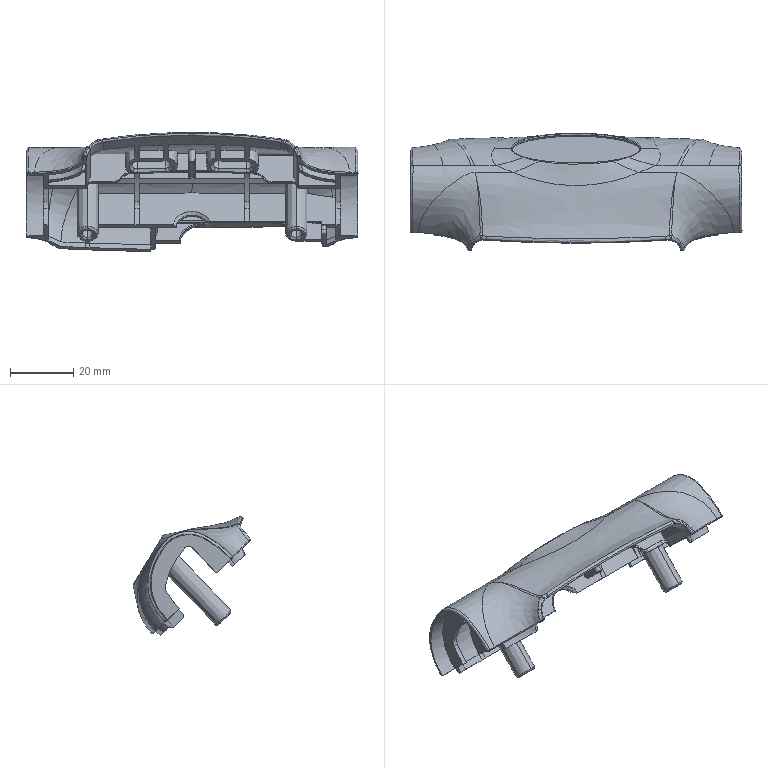Part | SolidWorks | features BaseBody 1 | 1 solid | 415 faces | box 104.995 x 37.214 x 37.691 mm | volume 20077 mm3 | spline 206 | plane 119 | cylinder 70 | cone 20 | commonest cylinder face diameters 0.6 x16 3.3 x8 50.022 x7 17.297 x5 3.4 x4 6.401 x4